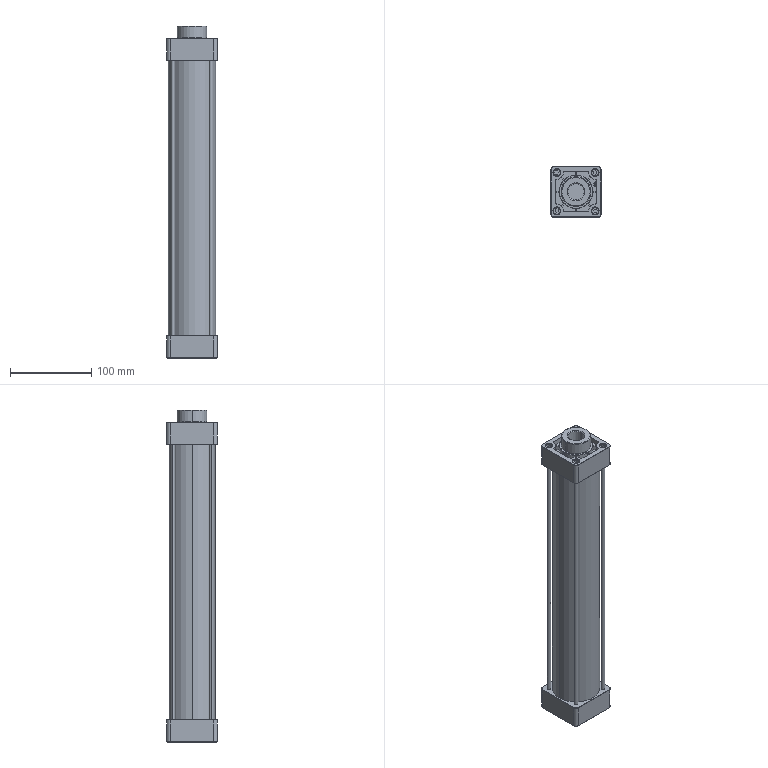Part | SolidWorks | 2 solids | 614 faces | box 62 x 62 x 408 mm | volume 454706 mm3 | plane 296 | spline 136 | cylinder 112 | cone 44 | torus 26 | commonest cylinder face diameters 12.301 x30 8.6 x16 9 x16 2 x10 4.5 x8 8 x8